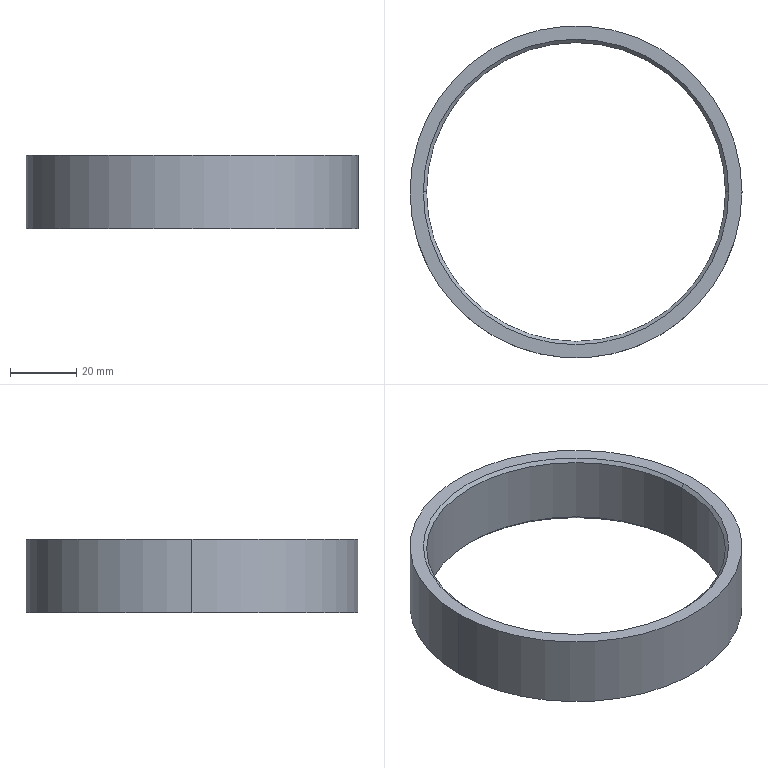Part | STEP file | 02-Spacer | 1 solid | 10 faces | box 100 x 100 x 22 mm | volume 32545 mm3 | cone 4 | cylinder 4 | plane 2 | commonest cylinder face diameters 90 x2 100 x2
STEP:
#1=CARTESIAN_POINT('',(0.,0.,0.));
#2=DIRECTION('',(0.,0.,1.));
#3=DIRECTION('',(1.,0.,0.));
#4=AXIS2_PLACEMENT_3D('',#1,#2,#3);
#5=CARTESIAN_POINT('',(45.,0.,21.));
#6=VERTEX_POINT('',#5);
#7=CARTESIAN_POINT('',(46.,0.,22.));
#8=VERTEX_POINT('',#7);
#9=CARTESIAN_POINT('',(45.,0.,21.));
#10=DIRECTION('',(0.7071,0.,0.7071));
#11=VECTOR('',#10,1.);
#12=LINE('',#9,#11);
#13=CARTESIAN_POINT('',(0.,0.,21.));
#14=DIRECTION('',(0.,0.,1.));
#15=DIRECTION('',(1.,0.,0.));
#16=AXIS2_PLACEMENT_3D('',#13,#14,#15);
#17=CONICAL_SURFACE('',#16,45.,0.7854);
#18=CARTESIAN_POINT('',(6.283,0.));
#19=DIRECTION('',(0.,1.));
#20=VECTOR('',#19,1.);
#21=LINE('',#18,#20);
#22=(GEOMETRIC_REPRESENTATION_CONTEXT(2)PARAMETRIC_REPRESENTATION_CONTEXT()REPRESENTATION_CONTEXT('',''));
#23=DEFINITIONAL_REPRESENTATION('',(#21),#22);
#24=PCURVE('',#17,#23);
#25=CARTESIAN_POINT('',(0.,0.,21.));
#26=DIRECTION('',(0.,0.,1.));
#27=DIRECTION('',(1.,0.,0.));
#28=AXIS2_PLACEMENT_3D('',#25,#26,#27);
#29=CONICAL_SURFACE('',#28,45.,0.7854);
#30=CARTESIAN_POINT('',(0.,0.));
#31=DIRECTION('',(0.,1.));
#32=VECTOR('',#31,1.);
#33=LINE('',#30,#32);
#34=(GEOMETRIC_REPRESENTATION_CONTEXT(2)PARAMETRIC_REPRESENTATION_CONTEXT()REPRESENTATION_CONTEXT('',''));
#35=DEFINITIONAL_REPRESENTATION('',(#33),#34);
#36=PCURVE('',#29,#35);
#37=SURFACE_CURVE('',#12,(#24,#36),.PCURVE_S1.);
#38=EDGE_CURVE('',#6,#8,#37,.T.);
#39=ORIENTED_EDGE('',*,*,#38,.T.);
#40=CARTESIAN_POINT('',(-46.,0.,22.));
#41=VERTEX_POINT('',#40);
#42=CARTESIAN_POINT('',(0.,0.,22.));
#43=DIRECTION('',(0.,0.,-1.));
#44=DIRECTION('',(1.,0.,0.));
#45=AXIS2_PLACEMENT_3D('',#42,#43,#44);
#46=CIRCLE('',#45,46.);
#47=CARTESIAN_POINT('',(6.283,1.));
#48=DIRECTION('',(-1.,0.));
#49=VECTOR('',#48,1.);
#50=LINE('',#47,#49);
#51=(GEOMETRIC_REPRESENTATION_CONTEXT(2)PARAMETRIC_REPRESENTATION_CONTEXT()REPRESENTATION_CONTEXT('',''));
#52=DEFINITIONAL_REPRESENTATION('',(#50),#51);
#53=PCURVE('',#17,#52);
#54=CARTESIAN_POINT('',(0.,0.,22.));
#55=DIRECTION('',(0.,0.,1.));
#56=DIRECTION('',(1.,0.,0.));
#57=AXIS2_PLACEMENT_3D('',#54,#55,#56);
#58=PLANE('',#57);
#59=CARTESIAN_POINT('',(46.,0.));
#60=CARTESIAN_POINT('',(46.,-79.674));
#61=CARTESIAN_POINT('',(-23.,-39.837));
#62=CARTESIAN_POINT('',(-92.,0.));
#63=CARTESIAN_POINT('',(-23.,39.837));
#64=CARTESIAN_POINT('',(46.,79.674));
#65=CARTESIAN_POINT('',(46.,0.));
#66=(BOUNDED_CURVE()B_SPLINE_CURVE(2,(#59,#60,#61,#62,#63,#64,#65),.UNSPECIFIED.,.T.,.F.)B_SPLINE_CURVE_WITH_KNOTS((1,2,2,2,2,1),(-2.094,0.,2.094,4.189,6.283,8.378),.UNSPECIFIED.)CURVE()GEOMETRIC_REPRESENTATION_ITEM()RATIONAL_B_SPLINE_CURVE((1.,0.5,1.,0.5,1.,0.5,1.))REPRESENTATION_ITEM(''));
#67=(GEOMETRIC_REPRESENTATION_CONTEXT(2)PARAMETRIC_REPRESENTATION_CONTEXT()REPRESENTATION_CONTEXT('',''));
#68=DEFINITIONAL_REPRESENTATION('',(#66),#67);
#69=PCURVE('',#58,#68);
#70=SURFACE_CURVE('',#46,(#53,#69),.PCURVE_S1.);
#71=EDGE_CURVE('',#8,#41,#70,.T.);
#72=ORIENTED_EDGE('',*,*,#71,.T.);
#73=CARTESIAN_POINT('',(-45.,0.,21.));
#74=VERTEX_POINT('',#73);
#75=CARTESIAN_POINT('',(-45.,0.,21.));
#76=DIRECTION('',(-0.7071,0.,0.7071));
#77=VECTOR('',#76,1.);
#78=LINE('',#75,#77);
#79=CARTESIAN_POINT('',(3.142,0.));
#80=DIRECTION('',(0.,1.));
#81=VECTOR('',#80,1.);
#82=LINE('',#79,#81);
#83=(GEOMETRIC_REPRESENTATION_CONTEXT(2)PARAMETRIC_REPRESENTATION_CONTEXT()REPRESENTATION_CONTEXT('',''));
#84=DEFINITIONAL_REPRESENTATION('',(#82),#83);
#85=PCURVE('',#17,#84);
#86=CARTESIAN_POINT('',(3.142,0.));
#87=DIRECTION('',(0.,1.));
#88=VECTOR('',#87,1.);
#89=LINE('',#86,#88);
#90=(GEOMETRIC_REPRESENTATION_CONTEXT(2)PARAMETRIC_REPRESENTATION_CONTEXT()REPRESENTATION_CONTEXT('',''));
#91=DEFINITIONAL_REPRESENTATION('',(#89),#90);
#92=PCURVE('',#29,#91);
#93=SURFACE_CURVE('',#78,(#85,#92),.PCURVE_S1.);
#94=EDGE_CURVE('',#74,#41,#93,.T.);
#95=ORIENTED_EDGE('',*,*,#94,.F.);
#96=CARTESIAN_POINT('',(0.,0.,21.));
#97=DIRECTION('',(0.,0.,1.));
#98=DIRECTION('',(1.,0.,0.));
#99=AXIS2_PLACEMENT_3D('',#96,#97,#98);
#100=CIRCLE('',#99,45.);
#101=CARTESIAN_POINT('',(0.,0.));
#102=DIRECTION('',(1.,0.));
#103=VECTOR('',#102,1.);
#104=LINE('',#101,#103);
#105=(GEOMETRIC_REPRESENTATION_CONTEXT(2)PARAMETRIC_REPRESENTATION_CONTEXT()REPRESENTATION_CONTEXT('',''));
#106=DEFINITIONAL_REPRESENTATION('',(#104),#105);
#107=PCURVE('',#17,#106);
#108=CARTESIAN_POINT('',(0.,0.,22.));
#109=DIRECTION('',(0.,0.,-1.));
#110=DIRECTION('',(-1.,0.,0.));
#111=AXIS2_PLACEMENT_3D('',#108,#109,#110);
#112=CYLINDRICAL_SURFACE('',#111,45.);
#113=CARTESIAN_POINT('',(9.425,1.));
#114=DIRECTION('',(-1.,0.));
#115=VECTOR('',#114,1.);
#116=LINE('',#113,#115);
#117=(GEOMETRIC_REPRESENTATION_CONTEXT(2)PARAMETRIC_REPRESENTATION_CONTEXT()REPRESENTATION_CONTEXT('',''));
#118=DEFINITIONAL_REPRESENTATION('',(#116),#117);
#119=PCURVE('',#112,#118);
#120=SURFACE_CURVE('',#100,(#107,#119),.PCURVE_S1.);
#121=EDGE_CURVE('',#74,#6,#120,.T.);
#122=ORIENTED_EDGE('',*,*,#121,.T.);
#123=EDGE_LOOP('',(#39,#72,#95,#122));
#124=FACE_BOUND('',#123,.F.);
#125=ADVANCED_FACE('',(#124),#17,.F.);
#126=CARTESIAN_POINT('',(-45.,0.,1.));
#127=VERTEX_POINT('',#126);
#128=CARTESIAN_POINT('',(-46.,0.,0.));
#129=VERTEX_POINT('',#128);
#130=CARTESIAN_POINT('',(-46.,0.,0.));
#131=DIRECTION('',(-0.7071,0.,-0.7071));
#132=VECTOR('',#131,1.);
#133=LINE('',#130,#132);
#134=CARTESIAN_POINT('',(0.,0.,0.));
#135=DIRECTION('',(0.,0.,-1.));
#136=DIRECTION('',(-1.,0.,0.));
#137=AXIS2_PLACEMENT_3D('',#134,#135,#136);
#138=CONICAL_SURFACE('',#137,46.,0.7854);
#139=CARTESIAN_POINT('',(6.283,0.));
#140=DIRECTION('',(0.,1.));
#141=VECTOR('',#140,1.);
#142=LINE('',#139,#141);
#143=(GEOMETRIC_REPRESENTATION_CONTEXT(2)PARAMETRIC_REPRESENTATION_CONTEXT()REPRESENTATION_CONTEXT('',''));
#144=DEFINITIONAL_REPRESENTATION('',(#142),#143);
#145=PCURVE('',#138,#144);
#146=CARTESIAN_POINT('',(0.,0.,0.));
#147=DIRECTION('',(0.,0.,-1.));
#148=DIRECTION('',(-1.,0.,0.));
#149=AXIS2_PLACEMENT_3D('',#146,#147,#148);
#150=CONICAL_SURFACE('',#149,46.,0.7854);
#151=CARTESIAN_POINT('',(0.,0.));
#152=DIRECTION('',(0.,1.));
#153=VECTOR('',#152,1.);
#154=LINE('',#151,#153);
#155=(GEOMETRIC_REPRESENTATION_CONTEXT(2)PARAMETRIC_REPRESENTATION_CONTEXT()REPRESENTATION_CONTEXT('',''));
#156=DEFINITIONAL_REPRESENTATION('',(#154),#155);
#157=PCURVE('',#150,#156);
#158=SURFACE_CURVE('',#133,(#145,#157),.PCURVE_S1.);
#159=EDGE_CURVE('',#127,#129,#158,.T.);
#160=ORIENTED_EDGE('',*,*,#159,.T.);
#161=CARTESIAN_POINT('',(46.,0.,0.));
#162=VERTEX_POINT('',#161);
#163=CARTESIAN_POINT('',(0.,0.,0.));
#164=DIRECTION('',(0.,0.,1.));
#165=DIRECTION('',(1.,0.,0.));
#166=AXIS2_PLACEMENT_3D('',#163,#164,#165);
#167=CIRCLE('',#166,46.);
#168=CARTESIAN_POINT('',(9.425,0.));
#169=DIRECTION('',(-1.,0.));
#170=VECTOR('',#169,1.);
#171=LINE('',#168,#170);
#172=(GEOMETRIC_REPRESENTATION_CONTEXT(2)PARAMETRIC_REPRESENTATION_CONTEXT()REPRESENTATION_CONTEXT('',''));
#173=DEFINITIONAL_REPRESENTATION('',(#171),#172);
#174=PCURVE('',#138,#173);
#175=CARTESIAN_POINT('',(0.,0.,0.));
#176=DIRECTION('',(0.,0.,1.));
#177=DIRECTION('',(1.,0.,0.));
#178=AXIS2_PLACEMENT_3D('',#175,#176,#177);
#179=PLANE('',#178);
#180=CARTESIAN_POINT('',(0.,0.));
#181=DIRECTION('',(1.,0.));
#182=AXIS2_PLACEMENT_2D('',#180,#181);
#183=CIRCLE('',#182,46.);
#184=(GEOMETRIC_REPRESENTATION_CONTEXT(2)PARAMETRIC_REPRESENTATION_CONTEXT()REPRESENTATION_CONTEXT('',''));
#185=DEFINITIONAL_REPRESENTATION('',(#183),#184);
#186=PCURVE('',#179,#185);
#187=SURFACE_CURVE('',#167,(#174,#186),.PCURVE_S1.);
#188=EDGE_CURVE('',#129,#162,#187,.T.);
#189=ORIENTED_EDGE('',*,*,#188,.T.);
#190=CARTESIAN_POINT('',(45.,0.,1.));
#191=VERTEX_POINT('',#190);
#192=CARTESIAN_POINT('',(46.,0.,0.));
#193=DIRECTION('',(0.7071,0.,-0.7071));
#194=VECTOR('',#193,1.);
#195=LINE('',#192,#194);
#196=CARTESIAN_POINT('',(3.142,0.));
#197=DIRECTION('',(0.,1.));
#198=VECTOR('',#197,1.);
#199=LINE('',#196,#198);
#200=(GEOMETRIC_REPRESENTATION_CONTEXT(2)PARAMETRIC_REPRESENTATION_CONTEXT()REPRESENTATION_CONTEXT('',''));
#201=DEFINITIONAL_REPRESENTATION('',(#199),#200);
#202=PCURVE('',#138,#201);
#203=CARTESIAN_POINT('',(3.142,0.));
#204=DIRECTION('',(0.,1.));
#205=VECTOR('',#204,1.);
#206=LINE('',#203,#205);
#207=(GEOMETRIC_REPRESENTATION_CONTEXT(2)PARAMETRIC_REPRESENTATION_CONTEXT()REPRESENTATION_CONTEXT('',''));
#208=DEFINITIONAL_REPRESENTATION('',(#206),#207);
#209=PCURVE('',#150,#208);
#210=SURFACE_CURVE('',#195,(#202,#209),.PCURVE_S1.);
#211=EDGE_CURVE('',#191,#162,#210,.T.);
#212=ORIENTED_EDGE('',*,*,#211,.F.);
#213=CARTESIAN_POINT('',(0.,0.,1.));
#214=DIRECTION('',(0.,0.,-1.));
#215=DIRECTION('',(1.,0.,0.));
#216=AXIS2_PLACEMENT_3D('',#213,#214,#215);
#217=CIRCLE('',#216,45.);
#218=CARTESIAN_POINT('',(3.142,-1.));
#219=DIRECTION('',(1.,0.));
#220=VECTOR('',#219,1.);
#221=LINE('',#218,#220);
#222=(GEOMETRIC_REPRESENTATION_CONTEXT(2)PARAMETRIC_REPRESENTATION_CONTEXT()REPRESENTATION_CONTEXT('',''));
#223=DEFINITIONAL_REPRESENTATION('',(#221),#222);
#224=PCURVE('',#138,#223);
#225=CARTESIAN_POINT('',(3.142,21.));
#226=DIRECTION('',(1.,0.));
#227=VECTOR('',#226,1.);
#228=LINE('',#225,#227);
#229=(GEOMETRIC_REPRESENTATION_CONTEXT(2)PARAMETRIC_REPRESENTATION_CONTEXT()REPRESENTATION_CONTEXT('',''));
#230=DEFINITIONAL_REPRESENTATION('',(#228),#229);
#231=PCURVE('',#112,#230);
#232=SURFACE_CURVE('',#217,(#224,#231),.PCURVE_S1.);
#233=EDGE_CURVE('',#191,#127,#232,.T.);
#234=ORIENTED_EDGE('',*,*,#233,.T.);
#235=EDGE_LOOP('',(#160,#189,#212,#234));
#236=FACE_BOUND('',#235,.F.);
#237=ADVANCED_FACE('',(#236),#138,.F.);
#238=CARTESIAN_POINT('',(-45.,0.,22.));
#239=DIRECTION('',(0.,0.,-1.));
#240=VECTOR('',#239,1.);
#241=LINE('',#238,#240);
#242=CARTESIAN_POINT('',(6.283,0.));
#243=DIRECTION('',(0.,1.));
#244=VECTOR('',#243,1.);
#245=LINE('',#242,#244);
#246=(GEOMETRIC_REPRESENTATION_CONTEXT(2)PARAMETRIC_REPRESENTATION_CONTEXT()REPRESENTATION_CONTEXT('',''));
#247=DEFINITIONAL_REPRESENTATION('',(#245),#246);
#248=PCURVE('',#112,#247);
#249=CARTESIAN_POINT('',(0.,0.,22.));
#250=DIRECTION('',(0.,0.,-1.));
#251=DIRECTION('',(-1.,0.,0.));
#252=AXIS2_PLACEMENT_3D('',#249,#250,#251);
#253=CYLINDRICAL_SURFACE('',#252,45.);
#254=CARTESIAN_POINT('',(0.,0.));
#255=DIRECTION('',(0.,1.));
#256=VECTOR('',#255,1.);
#257=LINE('',#254,#256);
#258=(GEOMETRIC_REPRESENTATION_CONTEXT(2)PARAMETRIC_REPRESENTATION_CONTEXT()REPRESENTATION_CONTEXT('',''));
#259=DEFINITIONAL_REPRESENTATION('',(#257),#258);
#260=PCURVE('',#253,#259);
#261=SURFACE_CURVE('',#241,(#248,#260),.PCURVE_S1.);
#262=EDGE_CURVE('',#74,#127,#261,.T.);
#263=ORIENTED_EDGE('',*,*,#262,.T.);
#264=ORIENTED_EDGE('',*,*,#233,.F.);
#265=CARTESIAN_POINT('',(45.,0.,22.));
#266=DIRECTION('',(0.,0.,-1.));
#267=VECTOR('',#266,1.);
#268=LINE('',#265,#267);
#269=CARTESIAN_POINT('',(3.142,0.));
#270=DIRECTION('',(0.,1.));
#271=VECTOR('',#270,1.);
#272=LINE('',#269,#271);
#273=(GEOMETRIC_REPRESENTATION_CONTEXT(2)PARAMETRIC_REPRESENTATION_CONTEXT()REPRESENTATION_CONTEXT('',''));
#274=DEFINITIONAL_REPRESENTATION('',(#272),#273);
#275=PCURVE('',#112,#274);
#276=CARTESIAN_POINT('',(3.142,0.));
#277=DIRECTION('',(0.,1.));
#278=VECTOR('',#277,1.);
#279=LINE('',#276,#278);
#280=(GEOMETRIC_REPRESENTATION_CONTEXT(2)PARAMETRIC_REPRESENTATION_CONTEXT()REPRESENTATION_CONTEXT('',''));
#281=DEFINITIONAL_REPRESENTATION('',(#279),#280);
#282=PCURVE('',#253,#281);
#283=SURFACE_CURVE('',#268,(#275,#282),.PCURVE_S1.);
#284=EDGE_CURVE('',#6,#191,#283,.T.);
#285=ORIENTED_EDGE('',*,*,#284,.F.);
#286=ORIENTED_EDGE('',*,*,#121,.F.);
#287=EDGE_LOOP('',(#263,#264,#285,#286));
#288=FACE_BOUND('',#287,.F.);
#289=ADVANCED_FACE('',(#288),#112,.F.);
#290=CARTESIAN_POINT('',(50.,0.,22.));
#291=VERTEX_POINT('',#290);
#292=CARTESIAN_POINT('',(-50.,0.,22.));
#293=VERTEX_POINT('',#292);
#294=CARTESIAN_POINT('',(0.,0.,22.));
#295=DIRECTION('',(0.,0.,1.));
#296=DIRECTION('',(1.,0.,0.));
#297=AXIS2_PLACEMENT_3D('',#294,#295,#296);
#298=CIRCLE('',#297,50.);
#299=CARTESIAN_POINT('',(0.,0.,22.));
#300=DIRECTION('',(0.,0.,-1.));
#301=DIRECTION('',(-1.,0.,0.));
#302=AXIS2_PLACEMENT_3D('',#299,#300,#301);
#303=CYLINDRICAL_SURFACE('',#302,50.);
#304=CARTESIAN_POINT('',(3.142,0.));
#305=DIRECTION('',(-1.,0.));
#306=VECTOR('',#305,1.);
#307=LINE('',#304,#306);
#308=(GEOMETRIC_REPRESENTATION_CONTEXT(2)PARAMETRIC_REPRESENTATION_CONTEXT()REPRESENTATION_CONTEXT('',''));
#309=DEFINITIONAL_REPRESENTATION('',(#307),#308);
#310=PCURVE('',#303,#309);
#311=CARTESIAN_POINT('',(0.,0.));
#312=DIRECTION('',(1.,0.));
#313=AXIS2_PLACEMENT_2D('',#311,#312);
#314=CIRCLE('',#313,50.);
#315=(GEOMETRIC_REPRESENTATION_CONTEXT(2)PARAMETRIC_REPRESENTATION_CONTEXT()REPRESENTATION_CONTEXT('',''));
#316=DEFINITIONAL_REPRESENTATION('',(#314),#315);
#317=PCURVE('',#58,#316);
#318=SURFACE_CURVE('',#298,(#310,#317),.PCURVE_S1.);
#319=EDGE_CURVE('',#291,#293,#318,.T.);
#320=ORIENTED_EDGE('',*,*,#319,.F.);
#321=CARTESIAN_POINT('',(50.,0.,0.));
#322=VERTEX_POINT('',#321);
#323=CARTESIAN_POINT('',(50.,0.,22.));
#324=DIRECTION('',(0.,0.,-1.));
#325=VECTOR('',#324,1.);
#326=LINE('',#323,#325);
#327=CARTESIAN_POINT('',(3.142,0.));
#328=DIRECTION('',(0.,1.));
#329=VECTOR('',#328,1.);
#330=LINE('',#327,#329);
#331=(GEOMETRIC_REPRESENTATION_CONTEXT(2)PARAMETRIC_REPRESENTATION_CONTEXT()REPRESENTATION_CONTEXT('',''));
#332=DEFINITIONAL_REPRESENTATION('',(#330),#331);
#333=PCURVE('',#303,#332);
#334=CARTESIAN_POINT('',(0.,0.,22.));
#335=DIRECTION('',(0.,0.,-1.));
#336=DIRECTION('',(-1.,0.,0.));
#337=AXIS2_PLACEMENT_3D('',#334,#335,#336);
#338=CYLINDRICAL_SURFACE('',#337,50.);
#339=CARTESIAN_POINT('',(3.142,0.));
#340=DIRECTION('',(0.,1.));
#341=VECTOR('',#340,1.);
#342=LINE('',#339,#341);
#343=(GEOMETRIC_REPRESENTATION_CONTEXT(2)PARAMETRIC_REPRESENTATION_CONTEXT()REPRESENTATION_CONTEXT('',''));
#344=DEFINITIONAL_REPRESENTATION('',(#342),#343);
#345=PCURVE('',#338,#344);
#346=SURFACE_CURVE('',#326,(#333,#345),.PCURVE_S1.);
#347=EDGE_CURVE('',#291,#322,#346,.T.);
#348=ORIENTED_EDGE('',*,*,#347,.T.);
#349=CARTESIAN_POINT('',(-50.,0.,0.));
#350=VERTEX_POINT('',#349);
#351=CARTESIAN_POINT('',(0.,0.,0.));
#352=DIRECTION('',(0.,0.,1.));
#353=DIRECTION('',(1.,0.,0.));
#354=AXIS2_PLACEMENT_3D('',#351,#352,#353);
#355=CIRCLE('',#354,50.);
#356=CARTESIAN_POINT('',(3.142,22.));
#357=DIRECTION('',(-1.,0.));
#358=VECTOR('',#357,1.);
#359=LINE('',#356,#358);
#360=(GEOMETRIC_REPRESENTATION_CONTEXT(2)PARAMETRIC_REPRESENTATION_CONTEXT()REPRESENTATION_CONTEXT('',''));
#361=DEFINITIONAL_REPRESENTATION('',(#359),#360);
#362=PCURVE('',#303,#361);
#363=CARTESIAN_POINT('',(0.,0.));
#364=DIRECTION('',(1.,0.));
#365=AXIS2_PLACEMENT_2D('',#363,#364);
#366=CIRCLE('',#365,50.);
#367=(GEOMETRIC_REPRESENTATION_CONTEXT(2)PARAMETRIC_REPRESENTATION_CONTEXT()REPRESENTATION_CONTEXT('',''));
#368=DEFINITIONAL_REPRESENTATION('',(#366),#367);
#369=PCURVE('',#179,#368);
#370=SURFACE_CURVE('',#355,(#362,#369),.PCURVE_S1.);
#371=EDGE_CURVE('',#322,#350,#370,.T.);
#372=ORIENTED_EDGE('',*,*,#371,.T.);
#373=CARTESIAN_POINT('',(-50.,0.,22.));
#374=DIRECTION('',(0.,0.,-1.));
#375=VECTOR('',#374,1.);
#376=LINE('',#373,#375);
#377=CARTESIAN_POINT('',(0.,0.));
#378=DIRECTION('',(0.,1.));
#379=VECTOR('',#378,1.);
#380=LINE('',#377,#379);
#381=(GEOMETRIC_REPRESENTATION_CONTEXT(2)PARAMETRIC_REPRESENTATION_CONTEXT()REPRESENTATION_CONTEXT('',''));
#382=DEFINITIONAL_REPRESENTATION('',(#380),#381);
#383=PCURVE('',#303,#382);
#384=CARTESIAN_POINT('',(6.283,0.));
#385=DIRECTION('',(0.,1.));
#386=VECTOR('',#385,1.);
#387=LINE('',#384,#386);
#388=(GEOMETRIC_REPRESENTATION_CONTEXT(2)PARAMETRIC_REPRESENTATION_CONTEXT()REPRESENTATION_CONTEXT('',''));
#389=DEFINITIONAL_REPRESENTATION('',(#387),#388);
#390=PCURVE('',#338,#389);
#391=SURFACE_CURVE('',#376,(#383,#390),.PCURVE_S1.);
#392=EDGE_CURVE('',#293,#350,#391,.T.);
#393=ORIENTED_EDGE('',*,*,#392,.F.);
#394=EDGE_LOOP('',(#320,#348,#372,#393));
#395=FACE_BOUND('',#394,.T.);
#396=ADVANCED_FACE('',(#395),#303,.T.);
#397=ORIENTED_EDGE('',*,*,#71,.T.);
#398=CARTESIAN_POINT('',(0.,0.,22.));
#399=DIRECTION('',(0.,0.,-1.));
#400=DIRECTION('',(1.,0.,0.));
#401=AXIS2_PLACEMENT_3D('',#398,#399,#400);
#402=CIRCLE('',#401,46.);
#403=CARTESIAN_POINT('',(46.,0.));
#404=CARTESIAN_POINT('',(46.,-79.674));
#405=CARTESIAN_POINT('',(-23.,-39.837));
#406=CARTESIAN_POINT('',(-92.,0.));
#407=CARTESIAN_POINT('',(-23.,39.837));
#408=CARTESIAN_POINT('',(46.,79.674));
#409=CARTESIAN_POINT('',(46.,0.));
#410=(BOUNDED_CURVE()B_SPLINE_CURVE(2,(#403,#404,#405,#406,#407,#408,#409),.UNSPECIFIED.,.T.,.F.)B_SPLINE_CURVE_WITH_KNOTS((1,2,2,2,2,1),(-2.094,0.,2.094,4.189,6.283,8.378),.UNSPECIFIED.)CURVE()GEOMETRIC_REPRESENTATION_ITEM()RATIONAL_B_SPLINE_CURVE((1.,0.5,1.,0.5,1.,0.5,1.))REPRESENTATION_ITEM(''));
#411=(GEOMETRIC_REPRESENTATION_CONTEXT(2)PARAMETRIC_REPRESENTATION_CONTEXT()REPRESENTATION_CONTEXT('',''));
#412=DEFINITIONAL_REPRESENTATION('',(#410),#411);
#413=PCURVE('',#58,#412);
#414=CARTESIAN_POINT('',(6.283,1.));
#415=DIRECTION('',(-1.,0.));
#416=VECTOR('',#415,1.);
#417=LINE('',#414,#416);
#418=(GEOMETRIC_REPRESENTATION_CONTEXT(2)PARAMETRIC_REPRESENTATION_CONTEXT()REPRESENTATION_CONTEXT('',''));
#419=DEFINITIONAL_REPRESENTATION('',(#417),#418);
#420=PCURVE('',#29,#419);
#421=SURFACE_CURVE('',#402,(#413,#420),.PCURVE_S1.);
#422=EDGE_CURVE('',#41,#8,#421,.T.);
#423=ORIENTED_EDGE('',*,*,#422,.T.);
#424=EDGE_LOOP('',(#397,#423));
#425=FACE_BOUND('',#424,.T.);
#426=CARTESIAN_POINT('',(0.,0.,22.));
#427=DIRECTION('',(0.,0.,1.));
#428=DIRECTION('',(1.,0.,0.));
#429=AXIS2_PLACEMENT_3D('',#426,#427,#428);
#430=CIRCLE('',#429,50.);
#431=CARTESIAN_POINT('',(0.,0.));
#432=DIRECTION('',(1.,0.));
#433=AXIS2_PLACEMENT_2D('',#431,#432);
#434=CIRCLE('',#433,50.);
#435=(GEOMETRIC_REPRESENTATION_CONTEXT(2)PARAMETRIC_REPRESENTATION_CONTEXT()REPRESENTATION_CONTEXT('',''));
#436=DEFINITIONAL_REPRESENTATION('',(#434),#435);
#437=PCURVE('',#58,#436);
#438=CARTESIAN_POINT('',(9.425,0.));
#439=DIRECTION('',(-1.,0.));
#440=VECTOR('',#439,1.);
#441=LINE('',#438,#440);
#442=(GEOMETRIC_REPRESENTATION_CONTEXT(2)PARAMETRIC_REPRESENTATION_CONTEXT()REPRESENTATION_CONTEXT('',''));
#443=DEFINITIONAL_REPRESENTATION('',(#441),#442);
#444=PCURVE('',#338,#443);
#445=SURFACE_CURVE('',#430,(#437,#444),.PCURVE_S1.);
#446=EDGE_CURVE('',#293,#291,#445,.T.);
#447=ORIENTED_EDGE('',*,*,#446,.T.);
#448=ORIENTED_EDGE('',*,*,#319,.T.);
#449=EDGE_LOOP('',(#447,#448));
#450=FACE_BOUND('',#449,.T.);
#451=ADVANCED_FACE('',(#425,#450),#58,.T.);
#452=ORIENTED_EDGE('',*,*,#188,.T.);
#453=CARTESIAN_POINT('',(0.,0.,0.));
#454=DIRECTION('',(0.,0.,1.));
#455=DIRECTION('',(1.,0.,0.));
#456=AXIS2_PLACEMENT_3D('',#453,#454,#455);
#457=CIRCLE('',#456,46.);
#458=CARTESIAN_POINT('',(0.,0.));
#459=DIRECTION('',(1.,0.));
#460=AXIS2_PLACEMENT_2D('',#458,#459);
#461=CIRCLE('',#460,46.);
#462=(GEOMETRIC_REPRESENTATION_CONTEXT(2)PARAMETRIC_REPRESENTATION_CONTEXT()REPRESENTATION_CONTEXT('',''));
#463=DEFINITIONAL_REPRESENTATION('',(#461),#462);
#464=PCURVE('',#179,#463);
#465=CARTESIAN_POINT('',(3.142,0.));
#466=DIRECTION('',(-1.,0.));
#467=VECTOR('',#466,1.);
#468=LINE('',#465,#467);
#469=(GEOMETRIC_REPRESENTATION_CONTEXT(2)PARAMETRIC_REPRESENTATION_CONTEXT()REPRESENTATION_CONTEXT('',''));
#470=DEFINITIONAL_REPRESENTATION('',(#468),#469);
#471=PCURVE('',#150,#470);
#472=SURFACE_CURVE('',#457,(#464,#471),.PCURVE_S1.);
#473=EDGE_CURVE('',#162,#129,#472,.T.);
#474=ORIENTED_EDGE('',*,*,#473,.T.);
#475=EDGE_LOOP('',(#452,#474));
#476=FACE_BOUND('',#475,.T.);
#477=CARTESIAN_POINT('',(0.,0.,0.));
#478=DIRECTION('',(0.,0.,1.));
#479=DIRECTION('',(1.,0.,0.));
#480=AXIS2_PLACEMENT_3D('',#477,#478,#479);
#481=CIRCLE('',#480,50.);
#482=CARTESIAN_POINT('',(0.,0.));
#483=DIRECTION('',(1.,0.));
#484=AXIS2_PLACEMENT_2D('',#482,#483);
#485=CIRCLE('',#484,50.);
#486=(GEOMETRIC_REPRESENTATION_CONTEXT(2)PARAMETRIC_REPRESENTATION_CONTEXT()REPRESENTATION_CONTEXT('',''));
#487=DEFINITIONAL_REPRESENTATION('',(#485),#486);
#488=PCURVE('',#179,#487);
#489=CARTESIAN_POINT('',(9.425,22.));
#490=DIRECTION('',(-1.,0.));
#491=VECTOR('',#490,1.);
#492=LINE('',#489,#491);
#493=(GEOMETRIC_REPRESENTATION_CONTEXT(2)PARAMETRIC_REPRESENTATION_CONTEXT()REPRESENTATION_CONTEXT('',''));
#494=DEFINITIONAL_REPRESENTATION('',(#492),#493);
#495=PCURVE('',#338,#494);
#496=SURFACE_CURVE('',#481,(#488,#495),.PCURVE_S1.);
#497=EDGE_CURVE('',#350,#322,#496,.T.);
#498=ORIENTED_EDGE('',*,*,#497,.F.);
#499=ORIENTED_EDGE('',*,*,#371,.F.);
#500=EDGE_LOOP('',(#498,#499));
#501=FACE_BOUND('',#500,.T.);
#502=ADVANCED_FACE('',(#476,#501),#179,.F.);
#503=ORIENTED_EDGE('',*,*,#347,.F.);
#504=ORIENTED_EDGE('',*,*,#446,.F.);
#505=ORIENTED_EDGE('',*,*,#392,.T.);
#506=ORIENTED_EDGE('',*,*,#497,.T.);
#507=EDGE_LOOP('',(#503,#504,#505,#506));
#508=FACE_BOUND('',#507,.T.);
#509=ADVANCED_FACE('',(#508),#338,.T.);
#510=CARTESIAN_POINT('',(0.,0.,1.));
#511=DIRECTION('',(0.,0.,-1.));
#512=DIRECTION('',(1.,0.,0.));
#513=AXIS2_PLACEMENT_3D('',#510,#511,#512);
#514=CIRCLE('',#513,45.);
#515=CARTESIAN_POINT('',(-3.142,21.));
#516=DIRECTION('',(1.,0.));
#517=VECTOR('',#516,1.);
#518=LINE('',#515,#517);
#519=(GEOMETRIC_REPRESENTATION_CONTEXT(2)PARAMETRIC_REPRESENTATION_CONTEXT()REPRESENTATION_CONTEXT('',''));
#520=DEFINITIONAL_REPRESENTATION('',(#518),#519);
#521=PCURVE('',#253,#520);
#522=CARTESIAN_POINT('',(-3.142,-1.));
#523=DIRECTION('',(1.,0.));
#524=VECTOR('',#523,1.);
#525=LINE('',#522,#524);
#526=(GEOMETRIC_REPRESENTATION_CONTEXT(2)PARAMETRIC_REPRESENTATION_CONTEXT()REPRESENTATION_CONTEXT('',''));
#527=DEFINITIONAL_REPRESENTATION('',(#525),#526);
#528=PCURVE('',#150,#527);
#529=SURFACE_CURVE('',#514,(#521,#528),.PCURVE_S1.);
#530=EDGE_CURVE('',#127,#191,#529,.T.);
#531=ORIENTED_EDGE('',*,*,#530,.F.);
#532=ORIENTED_EDGE('',*,*,#262,.F.);
#533=CARTESIAN_POINT('',(0.,0.,21.));
#534=DIRECTION('',(0.,0.,1.));
#535=DIRECTION('',(1.,0.,0.));
#536=AXIS2_PLACEMENT_3D('',#533,#534,#535);
#537=CIRCLE('',#536,45.);
#538=CARTESIAN_POINT('',(3.142,1.));
#539=DIRECTION('',(-1.,0.));
#540=VECTOR('',#539,1.);
#541=LINE('',#538,#540);
#542=(GEOMETRIC_REPRESENTATION_CONTEXT(2)PARAMETRIC_REPRESENTATION_CONTEXT()REPRESENTATION_CONTEXT('',''));
#543=DEFINITIONAL_REPRESENTATION('',(#541),#542);
#544=PCURVE('',#253,#543);
#545=CARTESIAN_POINT('',(0.,0.));
#546=DIRECTION('',(1.,0.));
#547=VECTOR('',#546,1.);
#548=LINE('',#545,#547);
#549=(GEOMETRIC_REPRESENTATION_CONTEXT(2)PARAMETRIC_REPRESENTATION_CONTEXT()REPRESENTATION_CONTEXT('',''));
#550=DEFINITIONAL_REPRESENTATION('',(#548),#549);
#551=PCURVE('',#29,#550);
#552=SURFACE_CURVE('',#537,(#544,#551),.PCURVE_S1.);
#553=EDGE_CURVE('',#6,#74,#552,.T.);
#554=ORIENTED_EDGE('',*,*,#553,.F.);
#555=ORIENTED_EDGE('',*,*,#284,.T.);
#556=EDGE_LOOP('',(#531,#532,#554,#555));
#557=FACE_BOUND('',#556,.F.);
#558=ADVANCED_FACE('',(#557),#253,.F.);
#559=ORIENTED_EDGE('',*,*,#473,.T.);
#560=ORIENTED_EDGE('',*,*,#159,.F.);
#561=ORIENTED_EDGE('',*,*,#530,.T.);
#562=ORIENTED_EDGE('',*,*,#211,.T.);
#563=EDGE_LOOP('',(#559,#560,#561,#562));
#564=FACE_BOUND('',#563,.F.);
#565=ADVANCED_FACE('',(#564),#150,.F.);
#566=ORIENTED_EDGE('',*,*,#422,.T.);
#567=ORIENTED_EDGE('',*,*,#38,.F.);
#568=ORIENTED_EDGE('',*,*,#553,.T.);
#569=ORIENTED_EDGE('',*,*,#94,.T.);
#570=EDGE_LOOP('',(#566,#567,#568,#569));
#571=FACE_BOUND('',#570,.F.);
#572=ADVANCED_FACE('',(#571),#29,.F.);
#573=CLOSED_SHELL('',(#125,#237,#289,#396,#451,#502,#509,#558,#565,#572));
#574=MANIFOLD_SOLID_BREP('',#573);
#575=(LENGTH_UNIT()NAMED_UNIT(*)SI_UNIT(.MILLI.,.METRE.));
#576=UNCERTAINTY_MEASURE_WITH_UNIT(LENGTH_MEASURE(0.0000001),#575,'','');
#577=(NAMED_UNIT(*)PLANE_ANGLE_UNIT()SI_UNIT($,.RADIAN.));
#578=(NAMED_UNIT(*)SI_UNIT($,.STERADIAN.)SOLID_ANGLE_UNIT());
#579=(GEOMETRIC_REPRESENTATION_CONTEXT(3)GLOBAL_UNCERTAINTY_ASSIGNED_CONTEXT((#576))GLOBAL_UNIT_ASSIGNED_CONTEXT((#575,#577,#578))REPRESENTATION_CONTEXT('',''));
#580=ADVANCED_BREP_SHAPE_REPRESENTATION('',(#4,#574),#579);